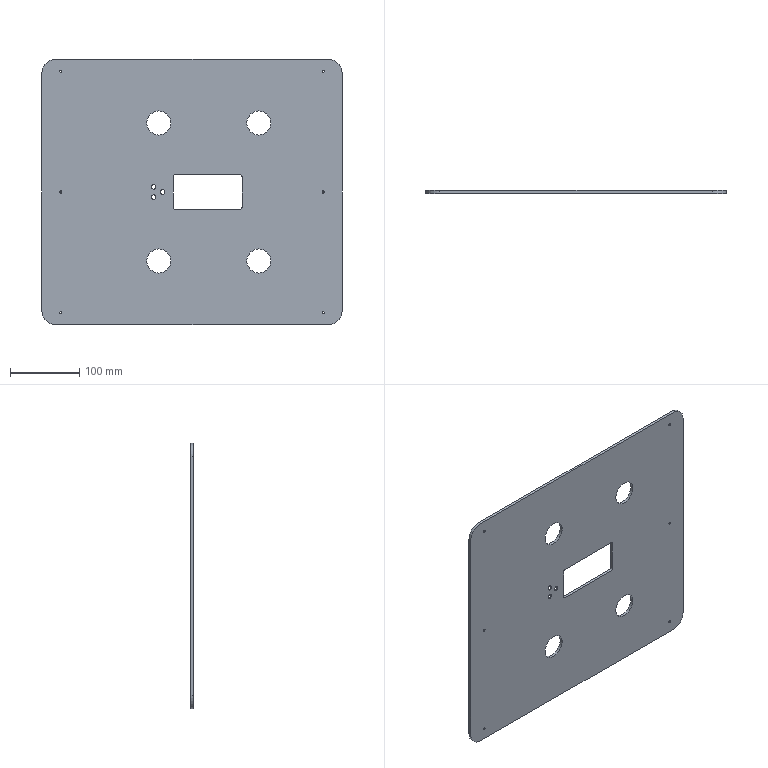Part | SolidWorks | features Cut 4, Extrusion 1, Fillet 1, HoleWzd 1 | 1 solid | 50 faces | box 435 x 4 x 385 mm | volume 632168 mm3 | cylinder 34 | plane 10 | cone 6 | commonest cylinder face diameters 3.2 x12 35 x8 6.6 x6 6 x4 40 x4